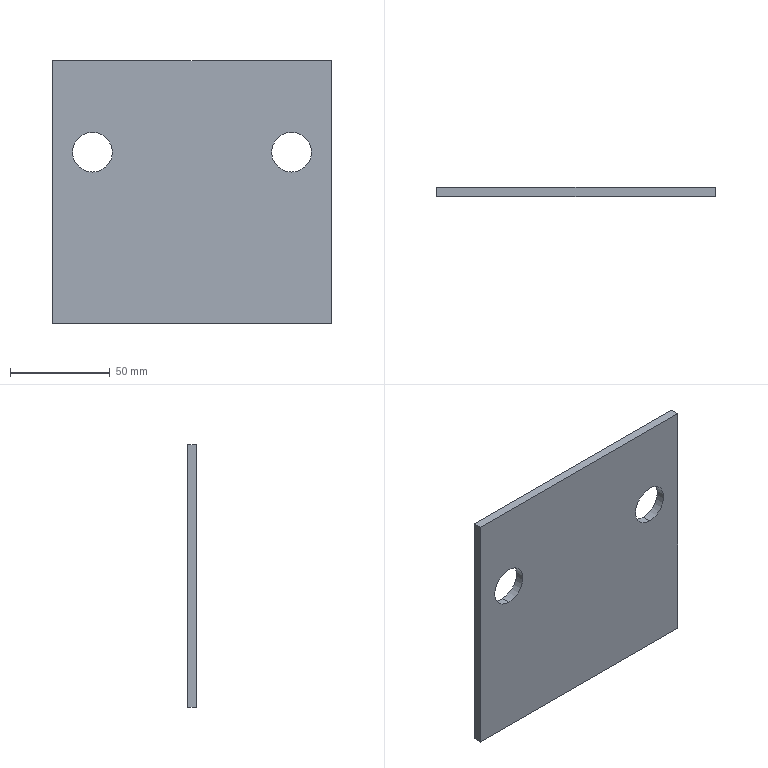Part | SolidWorks | features FlatPattern 1, SMBaseFlange 1, SheetMetal 1 | 1 solid | 10 faces | box 140 x 4.5 x 132 mm | volume 80333 mm3 | plane 6 | cylinder 4 | commonest cylinder face diameters 20 x4
STEP:
#1=CARTESIAN_POINT('',(120.,-4.5,76.));
#2=VERTEX_POINT('',#1);
#3=CARTESIAN_POINT('',(120.,-4.5,96.));
#4=VERTEX_POINT('',#3);
#5=CARTESIAN_POINT('',(120.,-4.5,86.));
#6=DIRECTION('',(0.,1.,0.));
#7=DIRECTION('',(0.,0.,1.));
#8=AXIS2_PLACEMENT_3D('',#5,#6,#7);
#9=CIRCLE('',#8,10.);
#10=EDGE_CURVE('',#2,#4,#9,.T.);
#11=ORIENTED_EDGE('',*,*,#10,.F.);
#12=CARTESIAN_POINT('',(120.,0.,76.));
#13=VERTEX_POINT('',#12);
#14=CARTESIAN_POINT('',(120.,-4.5,76.));
#15=DIRECTION('',(0.,1.,0.));
#16=VECTOR('',#15,1000.);
#17=LINE('',#14,#16);
#18=EDGE_CURVE('',#2,#13,#17,.T.);
#19=ORIENTED_EDGE('',*,*,#18,.T.);
#20=CARTESIAN_POINT('',(120.,0.,96.));
#21=VERTEX_POINT('',#20);
#22=CARTESIAN_POINT('',(120.,0.,86.));
#23=DIRECTION('',(0.,1.,0.));
#24=DIRECTION('',(0.,0.,1.));
#25=AXIS2_PLACEMENT_3D('',#22,#23,#24);
#26=CIRCLE('',#25,10.);
#27=EDGE_CURVE('',#13,#21,#26,.T.);
#28=ORIENTED_EDGE('',*,*,#27,.T.);
#29=CARTESIAN_POINT('',(120.,-4.5,96.));
#30=DIRECTION('',(0.,1.,0.));
#31=VECTOR('',#30,1000.);
#32=LINE('',#29,#31);
#33=EDGE_CURVE('',#4,#21,#32,.T.);
#34=ORIENTED_EDGE('',*,*,#33,.F.);
#35=EDGE_LOOP('',(#11,#19,#28,#34));
#36=FACE_OUTER_BOUND('',#35,.T.);
#37=CARTESIAN_POINT('',(120.,-4.5,86.));
#38=DIRECTION('',(0.,1.,0.));
#39=DIRECTION('',(0.,0.,1.));
#40=AXIS2_PLACEMENT_3D('',#37,#38,#39);
#41=CYLINDRICAL_SURFACE('',#40,10.);
#42=ADVANCED_FACE('',(#36),#41,.F.);
#43=CARTESIAN_POINT('',(20.,-4.5,76.));
#44=VERTEX_POINT('',#43);
#45=CARTESIAN_POINT('',(20.,-4.5,96.));
#46=VERTEX_POINT('',#45);
#47=CARTESIAN_POINT('',(20.,-4.5,86.));
#48=DIRECTION('',(0.,1.,0.));
#49=DIRECTION('',(0.,0.,1.));
#50=AXIS2_PLACEMENT_3D('',#47,#48,#49);
#51=CIRCLE('',#50,10.);
#52=EDGE_CURVE('',#44,#46,#51,.T.);
#53=ORIENTED_EDGE('',*,*,#52,.F.);
#54=CARTESIAN_POINT('',(20.,0.,76.));
#55=VERTEX_POINT('',#54);
#56=CARTESIAN_POINT('',(20.,-4.5,76.));
#57=DIRECTION('',(0.,1.,0.));
#58=VECTOR('',#57,1000.);
#59=LINE('',#56,#58);
#60=EDGE_CURVE('',#44,#55,#59,.T.);
#61=ORIENTED_EDGE('',*,*,#60,.T.);
#62=CARTESIAN_POINT('',(20.,0.,96.));
#63=VERTEX_POINT('',#62);
#64=CARTESIAN_POINT('',(20.,0.,86.));
#65=DIRECTION('',(0.,1.,0.));
#66=DIRECTION('',(0.,0.,1.));
#67=AXIS2_PLACEMENT_3D('',#64,#65,#66);
#68=CIRCLE('',#67,10.);
#69=EDGE_CURVE('',#55,#63,#68,.T.);
#70=ORIENTED_EDGE('',*,*,#69,.T.);
#71=CARTESIAN_POINT('',(20.,-4.5,96.));
#72=DIRECTION('',(0.,1.,0.));
#73=VECTOR('',#72,1000.);
#74=LINE('',#71,#73);
#75=EDGE_CURVE('',#46,#63,#74,.T.);
#76=ORIENTED_EDGE('',*,*,#75,.F.);
#77=EDGE_LOOP('',(#53,#61,#70,#76));
#78=FACE_OUTER_BOUND('',#77,.T.);
#79=CARTESIAN_POINT('',(20.,-4.5,86.));
#80=DIRECTION('',(0.,1.,0.));
#81=DIRECTION('',(0.,0.,1.));
#82=AXIS2_PLACEMENT_3D('',#79,#80,#81);
#83=CYLINDRICAL_SURFACE('',#82,10.);
#84=ADVANCED_FACE('',(#78),#83,.F.);
#85=CARTESIAN_POINT('',(0.,0.,0.));
#86=VERTEX_POINT('',#85);
#87=CARTESIAN_POINT('',(0.,0.,132.));
#88=VERTEX_POINT('',#87);
#89=CARTESIAN_POINT('',(0.,0.,0.));
#90=DIRECTION('',(0.,0.,1.));
#91=VECTOR('',#90,1000.);
#92=LINE('',#89,#91);
#93=EDGE_CURVE('',#86,#88,#92,.T.);
#94=ORIENTED_EDGE('',*,*,#93,.F.);
#95=CARTESIAN_POINT('',(0.,-4.5,0.));
#96=VERTEX_POINT('',#95);
#97=CARTESIAN_POINT('',(0.,-4.5,0.));
#98=DIRECTION('',(0.,1.,0.));
#99=VECTOR('',#98,1000.);
#100=LINE('',#97,#99);
#101=EDGE_CURVE('',#96,#86,#100,.T.);
#102=ORIENTED_EDGE('',*,*,#101,.F.);
#103=CARTESIAN_POINT('',(0.,-4.5,132.));
#104=VERTEX_POINT('',#103);
#105=CARTESIAN_POINT('',(0.,-4.5,0.));
#106=DIRECTION('',(0.,0.,1.));
#107=VECTOR('',#106,1000.);
#108=LINE('',#105,#107);
#109=EDGE_CURVE('',#96,#104,#108,.T.);
#110=ORIENTED_EDGE('',*,*,#109,.T.);
#111=CARTESIAN_POINT('',(0.,-4.5,132.));
#112=DIRECTION('',(0.,1.,0.));
#113=VECTOR('',#112,1000.);
#114=LINE('',#111,#113);
#115=EDGE_CURVE('',#104,#88,#114,.T.);
#116=ORIENTED_EDGE('',*,*,#115,.T.);
#117=EDGE_LOOP('',(#94,#102,#110,#116));
#118=FACE_OUTER_BOUND('',#117,.T.);
#119=CARTESIAN_POINT('',(0.,-4.5,0.));
#120=DIRECTION('',(-1.,0.,0.));
#121=DIRECTION('',(0.,0.,1.));
#122=AXIS2_PLACEMENT_3D('',#119,#120,#121);
#123=PLANE('',#122);
#124=ADVANCED_FACE('',(#118),#123,.T.);
#125=CARTESIAN_POINT('',(140.,0.,0.));
#126=VERTEX_POINT('',#125);
#127=CARTESIAN_POINT('',(0.,0.,0.));
#128=DIRECTION('',(-1.,0.,0.));
#129=VECTOR('',#128,1000.);
#130=LINE('',#127,#129);
#131=EDGE_CURVE('',#126,#86,#130,.T.);
#132=ORIENTED_EDGE('',*,*,#131,.F.);
#133=CARTESIAN_POINT('',(140.,-4.5,0.));
#134=VERTEX_POINT('',#133);
#135=CARTESIAN_POINT('',(140.,-4.5,0.));
#136=DIRECTION('',(0.,1.,0.));
#137=VECTOR('',#136,1000.);
#138=LINE('',#135,#137);
#139=EDGE_CURVE('',#134,#126,#138,.T.);
#140=ORIENTED_EDGE('',*,*,#139,.F.);
#141=CARTESIAN_POINT('',(0.,-4.5,0.));
#142=DIRECTION('',(-1.,0.,0.));
#143=VECTOR('',#142,1000.);
#144=LINE('',#141,#143);
#145=EDGE_CURVE('',#134,#96,#144,.T.);
#146=ORIENTED_EDGE('',*,*,#145,.T.);
#147=ORIENTED_EDGE('',*,*,#101,.T.);
#148=EDGE_LOOP('',(#132,#140,#146,#147));
#149=FACE_OUTER_BOUND('',#148,.T.);
#150=CARTESIAN_POINT('',(0.,-4.5,0.));
#151=DIRECTION('',(0.,0.,-1.));
#152=DIRECTION('',(-1.,0.,0.));
#153=AXIS2_PLACEMENT_3D('',#150,#151,#152);
#154=PLANE('',#153);
#155=ADVANCED_FACE('',(#149),#154,.T.);
#156=CARTESIAN_POINT('',(140.,0.,132.));
#157=VERTEX_POINT('',#156);
#158=CARTESIAN_POINT('',(140.,0.,0.));
#159=DIRECTION('',(0.,0.,-1.));
#160=VECTOR('',#159,1000.);
#161=LINE('',#158,#160);
#162=EDGE_CURVE('',#157,#126,#161,.T.);
#163=ORIENTED_EDGE('',*,*,#162,.F.);
#164=CARTESIAN_POINT('',(140.,-4.5,132.));
#165=VERTEX_POINT('',#164);
#166=CARTESIAN_POINT('',(140.,-4.5,132.));
#167=DIRECTION('',(0.,1.,0.));
#168=VECTOR('',#167,1000.);
#169=LINE('',#166,#168);
#170=EDGE_CURVE('',#165,#157,#169,.T.);
#171=ORIENTED_EDGE('',*,*,#170,.F.);
#172=CARTESIAN_POINT('',(140.,-4.5,0.));
#173=DIRECTION('',(0.,0.,-1.));
#174=VECTOR('',#173,1000.);
#175=LINE('',#172,#174);
#176=EDGE_CURVE('',#165,#134,#175,.T.);
#177=ORIENTED_EDGE('',*,*,#176,.T.);
#178=ORIENTED_EDGE('',*,*,#139,.T.);
#179=EDGE_LOOP('',(#163,#171,#177,#178));
#180=FACE_OUTER_BOUND('',#179,.T.);
#181=CARTESIAN_POINT('',(140.,-4.5,0.));
#182=DIRECTION('',(1.,0.,0.));
#183=DIRECTION('',(0.,0.,-1.));
#184=AXIS2_PLACEMENT_3D('',#181,#182,#183);
#185=PLANE('',#184);
#186=ADVANCED_FACE('',(#180),#185,.T.);
#187=CARTESIAN_POINT('',(0.,0.,132.));
#188=DIRECTION('',(1.,0.,0.));
#189=VECTOR('',#188,1000.);
#190=LINE('',#187,#189);
#191=EDGE_CURVE('',#88,#157,#190,.T.);
#192=ORIENTED_EDGE('',*,*,#191,.F.);
#193=ORIENTED_EDGE('',*,*,#115,.F.);
#194=CARTESIAN_POINT('',(0.,-4.5,132.));
#195=DIRECTION('',(1.,0.,0.));
#196=VECTOR('',#195,1000.);
#197=LINE('',#194,#196);
#198=EDGE_CURVE('',#104,#165,#197,.T.);
#199=ORIENTED_EDGE('',*,*,#198,.T.);
#200=ORIENTED_EDGE('',*,*,#170,.T.);
#201=EDGE_LOOP('',(#192,#193,#199,#200));
#202=FACE_OUTER_BOUND('',#201,.T.);
#203=CARTESIAN_POINT('',(0.,-4.5,132.));
#204=DIRECTION('',(0.,0.,1.));
#205=DIRECTION('',(1.,0.,0.));
#206=AXIS2_PLACEMENT_3D('',#203,#204,#205);
#207=PLANE('',#206);
#208=ADVANCED_FACE('',(#202),#207,.T.);
#209=CARTESIAN_POINT('',(120.,-4.5,86.));
#210=DIRECTION('',(0.,1.,0.));
#211=DIRECTION('',(0.,0.,1.));
#212=AXIS2_PLACEMENT_3D('',#209,#210,#211);
#213=CIRCLE('',#212,10.);
#214=EDGE_CURVE('',#4,#2,#213,.T.);
#215=ORIENTED_EDGE('',*,*,#214,.T.);
#216=ORIENTED_EDGE('',*,*,#10,.T.);
#217=EDGE_LOOP('',(#215,#216));
#218=FACE_BOUND('',#217,.T.);
#219=CARTESIAN_POINT('',(20.,-4.5,86.));
#220=DIRECTION('',(0.,1.,0.));
#221=DIRECTION('',(0.,0.,1.));
#222=AXIS2_PLACEMENT_3D('',#219,#220,#221);
#223=CIRCLE('',#222,10.);
#224=EDGE_CURVE('',#46,#44,#223,.T.);
#225=ORIENTED_EDGE('',*,*,#224,.T.);
#226=ORIENTED_EDGE('',*,*,#52,.T.);
#227=EDGE_LOOP('',(#225,#226));
#228=FACE_BOUND('',#227,.T.);
#229=ORIENTED_EDGE('',*,*,#109,.F.);
#230=ORIENTED_EDGE('',*,*,#145,.F.);
#231=ORIENTED_EDGE('',*,*,#176,.F.);
#232=ORIENTED_EDGE('',*,*,#198,.F.);
#233=EDGE_LOOP('',(#229,#230,#231,#232));
#234=FACE_OUTER_BOUND('',#233,.T.);
#235=CARTESIAN_POINT('',(0.,-4.5,0.));
#236=DIRECTION('',(0.,1.,0.));
#237=DIRECTION('',(0.,0.,1.));
#238=AXIS2_PLACEMENT_3D('',#235,#236,#237);
#239=PLANE('',#238);
#240=ADVANCED_FACE('',(#218,#228,#234),#239,.F.);
#241=CARTESIAN_POINT('',(120.,0.,86.));
#242=DIRECTION('',(0.,1.,0.));
#243=DIRECTION('',(0.,0.,1.));
#244=AXIS2_PLACEMENT_3D('',#241,#242,#243);
#245=CIRCLE('',#244,10.);
#246=EDGE_CURVE('',#21,#13,#245,.T.);
#247=ORIENTED_EDGE('',*,*,#246,.F.);
#248=ORIENTED_EDGE('',*,*,#27,.F.);
#249=EDGE_LOOP('',(#247,#248));
#250=FACE_BOUND('',#249,.T.);
#251=CARTESIAN_POINT('',(20.,0.,86.));
#252=DIRECTION('',(0.,1.,0.));
#253=DIRECTION('',(0.,0.,1.));
#254=AXIS2_PLACEMENT_3D('',#251,#252,#253);
#255=CIRCLE('',#254,10.);
#256=EDGE_CURVE('',#63,#55,#255,.T.);
#257=ORIENTED_EDGE('',*,*,#256,.F.);
#258=ORIENTED_EDGE('',*,*,#69,.F.);
#259=EDGE_LOOP('',(#257,#258));
#260=FACE_BOUND('',#259,.T.);
#261=ORIENTED_EDGE('',*,*,#93,.T.);
#262=ORIENTED_EDGE('',*,*,#191,.T.);
#263=ORIENTED_EDGE('',*,*,#162,.T.);
#264=ORIENTED_EDGE('',*,*,#131,.T.);
#265=EDGE_LOOP('',(#261,#262,#263,#264));
#266=FACE_OUTER_BOUND('',#265,.T.);
#267=CARTESIAN_POINT('',(0.,0.,0.));
#268=DIRECTION('',(0.,1.,0.));
#269=DIRECTION('',(0.,0.,1.));
#270=AXIS2_PLACEMENT_3D('',#267,#268,#269);
#271=PLANE('',#270);
#272=ADVANCED_FACE('',(#250,#260,#266),#271,.T.);
#273=ORIENTED_EDGE('',*,*,#60,.F.);
#274=ORIENTED_EDGE('',*,*,#224,.F.);
#275=ORIENTED_EDGE('',*,*,#75,.T.);
#276=ORIENTED_EDGE('',*,*,#256,.T.);
#277=EDGE_LOOP('',(#273,#274,#275,#276));
#278=FACE_OUTER_BOUND('',#277,.T.);
#279=CARTESIAN_POINT('',(20.,-4.5,86.));
#280=DIRECTION('',(0.,1.,0.));
#281=DIRECTION('',(0.,0.,1.));
#282=AXIS2_PLACEMENT_3D('',#279,#280,#281);
#283=CYLINDRICAL_SURFACE('',#282,10.);
#284=ADVANCED_FACE('',(#278),#283,.F.);
#285=ORIENTED_EDGE('',*,*,#18,.F.);
#286=ORIENTED_EDGE('',*,*,#214,.F.);
#287=ORIENTED_EDGE('',*,*,#33,.T.);
#288=ORIENTED_EDGE('',*,*,#246,.T.);
#289=EDGE_LOOP('',(#285,#286,#287,#288));
#290=FACE_OUTER_BOUND('',#289,.T.);
#291=CARTESIAN_POINT('',(120.,-4.5,86.));
#292=DIRECTION('',(0.,1.,0.));
#293=DIRECTION('',(0.,0.,1.));
#294=AXIS2_PLACEMENT_3D('',#291,#292,#293);
#295=CYLINDRICAL_SURFACE('',#294,10.);
#296=ADVANCED_FACE('',(#290),#295,.F.);
#297=CLOSED_SHELL('',(#42,#84,#124,#155,#186,#208,#240,#272,#284,#296));
#298=MANIFOLD_SOLID_BREP('',#297);
#299=CARTESIAN_POINT('',(0.,0.,0.));
#300=DIRECTION('',(0.,0.,1.));
#301=DIRECTION('',(1.,0.,0.));
#302=AXIS2_PLACEMENT_3D('',#299,#300,#301);
#303=(LENGTH_UNIT()NAMED_UNIT(*)SI_UNIT(.MILLI.,.METRE.));
#304=UNCERTAINTY_MEASURE_WITH_UNIT(LENGTH_MEASURE(0.00001),#303,'','');
#305=(NAMED_UNIT(*)PLANE_ANGLE_UNIT()SI_UNIT($,.RADIAN.));
#306=(NAMED_UNIT(*)SI_UNIT($,.STERADIAN.)SOLID_ANGLE_UNIT());
#307=(GEOMETRIC_REPRESENTATION_CONTEXT(3)GLOBAL_UNCERTAINTY_ASSIGNED_CONTEXT((#304))GLOBAL_UNIT_ASSIGNED_CONTEXT((#303,#305,#306))REPRESENTATION_CONTEXT('',''));
#308=ADVANCED_BREP_SHAPE_REPRESENTATION('',(#298,#302),#307);